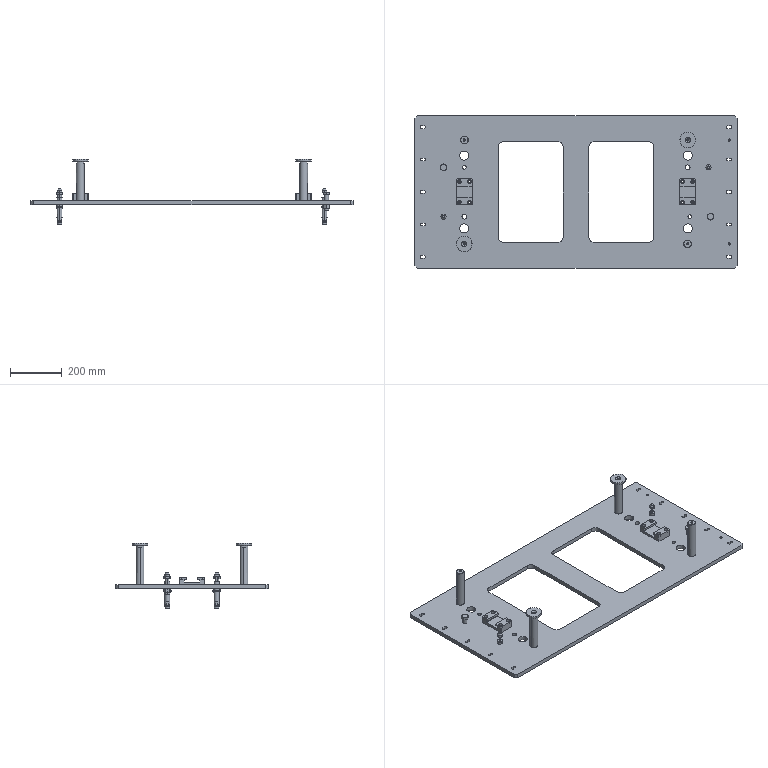Part | SolidWorks | 19 solids | 586 faces | box 1240 x 588 x 250.5 mm | volume 9199550 mm3 | cylinder 226 | plane 216 | cone 144 | commonest cylinder face diameters 11 x42 29.132 x28 8.5 x20 6.8 x16 9 x16 15 x16